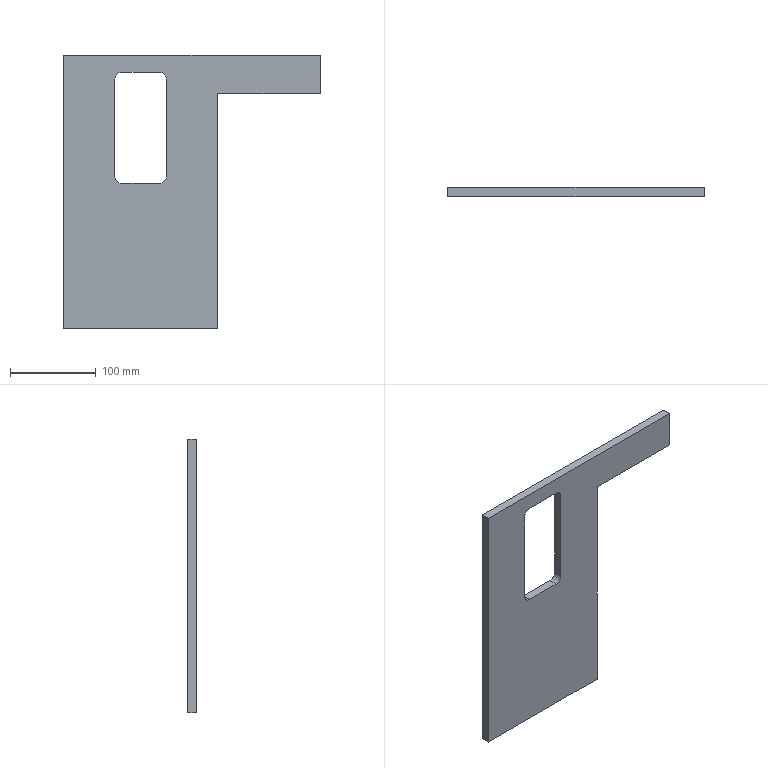Part | SolidWorks | features Cut 1, Extrusion 1, Fillet 1, ICE 1 | 1 solid | 16 faces | box 300 x 10 x 320 mm | volume 552549 mm3 | plane 12 | cylinder 4 | commonest cylinder face diameters 16 x4
STEP:
#1=CARTESIAN_POINT('',(90.,0.,115.));
#2=VERTEX_POINT('',#1);
#3=CARTESIAN_POINT('',(90.,10.,115.));
#4=VERTEX_POINT('',#3);
#5=CARTESIAN_POINT('',(90.,10.,115.));
#6=DIRECTION('',(0.,1.,0.));
#7=VECTOR('',#6,1000.);
#8=LINE('',#5,#7);
#9=EDGE_CURVE('',#2,#4,#8,.T.);
#10=ORIENTED_EDGE('',*,*,#9,.F.);
#11=CARTESIAN_POINT('',(90.,0.,-160.));
#12=VERTEX_POINT('',#11);
#13=CARTESIAN_POINT('',(90.,0.,-160.));
#14=DIRECTION('',(0.,0.,-1.));
#15=VECTOR('',#14,1000.);
#16=LINE('',#13,#15);
#17=EDGE_CURVE('',#2,#12,#16,.T.);
#18=ORIENTED_EDGE('',*,*,#17,.T.);
#19=CARTESIAN_POINT('',(90.,10.,-160.));
#20=VERTEX_POINT('',#19);
#21=CARTESIAN_POINT('',(90.,10.,-160.));
#22=DIRECTION('',(0.,-1.,0.));
#23=VECTOR('',#22,1000.);
#24=LINE('',#21,#23);
#25=EDGE_CURVE('',#20,#12,#24,.T.);
#26=ORIENTED_EDGE('',*,*,#25,.F.);
#27=CARTESIAN_POINT('',(90.,10.,-160.));
#28=DIRECTION('',(0.,0.,-1.));
#29=VECTOR('',#28,1000.);
#30=LINE('',#27,#29);
#31=EDGE_CURVE('',#4,#20,#30,.T.);
#32=ORIENTED_EDGE('',*,*,#31,.F.);
#33=EDGE_LOOP('',(#10,#18,#26,#32));
#34=FACE_OUTER_BOUND('',#33,.T.);
#35=CARTESIAN_POINT('',(90.,10.,-160.));
#36=DIRECTION('',(-1.,0.,0.));
#37=DIRECTION('',(0.,0.,1.));
#38=AXIS2_PLACEMENT_3D('',#35,#36,#37);
#39=PLANE('',#38);
#40=ADVANCED_FACE('',(#34),#39,.F.);
#41=CARTESIAN_POINT('',(-90.,0.,-160.));
#42=VERTEX_POINT('',#41);
#43=CARTESIAN_POINT('',(-90.,0.,-160.));
#44=DIRECTION('',(-1.,0.,0.));
#45=VECTOR('',#44,1000.);
#46=LINE('',#43,#45);
#47=EDGE_CURVE('',#12,#42,#46,.T.);
#48=ORIENTED_EDGE('',*,*,#47,.T.);
#49=CARTESIAN_POINT('',(-90.,10.,-160.));
#50=VERTEX_POINT('',#49);
#51=CARTESIAN_POINT('',(-90.,10.,-160.));
#52=DIRECTION('',(0.,-1.,0.));
#53=VECTOR('',#52,1000.);
#54=LINE('',#51,#53);
#55=EDGE_CURVE('',#50,#42,#54,.T.);
#56=ORIENTED_EDGE('',*,*,#55,.F.);
#57=CARTESIAN_POINT('',(-90.,10.,-160.));
#58=DIRECTION('',(-1.,0.,0.));
#59=VECTOR('',#58,1000.);
#60=LINE('',#57,#59);
#61=EDGE_CURVE('',#20,#50,#60,.T.);
#62=ORIENTED_EDGE('',*,*,#61,.F.);
#63=ORIENTED_EDGE('',*,*,#25,.T.);
#64=EDGE_LOOP('',(#48,#56,#62,#63));
#65=FACE_OUTER_BOUND('',#64,.T.);
#66=CARTESIAN_POINT('',(-90.,10.,-160.));
#67=DIRECTION('',(0.,0.,1.));
#68=DIRECTION('',(1.,0.,0.));
#69=AXIS2_PLACEMENT_3D('',#66,#67,#68);
#70=PLANE('',#69);
#71=ADVANCED_FACE('',(#65),#70,.F.);
#72=CARTESIAN_POINT('',(-90.,0.,160.));
#73=VERTEX_POINT('',#72);
#74=CARTESIAN_POINT('',(-90.,0.,-160.));
#75=DIRECTION('',(0.,0.,1.));
#76=VECTOR('',#75,1000.);
#77=LINE('',#74,#76);
#78=EDGE_CURVE('',#42,#73,#77,.T.);
#79=ORIENTED_EDGE('',*,*,#78,.T.);
#80=CARTESIAN_POINT('',(-90.,10.,160.));
#81=VERTEX_POINT('',#80);
#82=CARTESIAN_POINT('',(-90.,10.,160.));
#83=DIRECTION('',(0.,-1.,0.));
#84=VECTOR('',#83,1000.);
#85=LINE('',#82,#84);
#86=EDGE_CURVE('',#81,#73,#85,.T.);
#87=ORIENTED_EDGE('',*,*,#86,.F.);
#88=CARTESIAN_POINT('',(-90.,10.,-160.));
#89=DIRECTION('',(0.,0.,1.));
#90=VECTOR('',#89,1000.);
#91=LINE('',#88,#90);
#92=EDGE_CURVE('',#50,#81,#91,.T.);
#93=ORIENTED_EDGE('',*,*,#92,.F.);
#94=ORIENTED_EDGE('',*,*,#55,.T.);
#95=EDGE_LOOP('',(#79,#87,#93,#94));
#96=FACE_OUTER_BOUND('',#95,.T.);
#97=CARTESIAN_POINT('',(-90.,10.,-160.));
#98=DIRECTION('',(1.,0.,0.));
#99=DIRECTION('',(0.,0.,-1.));
#100=AXIS2_PLACEMENT_3D('',#97,#98,#99);
#101=PLANE('',#100);
#102=ADVANCED_FACE('',(#96),#101,.F.);
#103=CARTESIAN_POINT('',(210.,0.,160.));
#104=VERTEX_POINT('',#103);
#105=CARTESIAN_POINT('',(-90.,0.,160.));
#106=DIRECTION('',(1.,0.,0.));
#107=VECTOR('',#106,1000.);
#108=LINE('',#105,#107);
#109=EDGE_CURVE('',#73,#104,#108,.T.);
#110=ORIENTED_EDGE('',*,*,#109,.T.);
#111=CARTESIAN_POINT('',(210.,10.,160.));
#112=VERTEX_POINT('',#111);
#113=CARTESIAN_POINT('',(210.,10.,160.));
#114=DIRECTION('',(0.,-1.,0.));
#115=VECTOR('',#114,1000.);
#116=LINE('',#113,#115);
#117=EDGE_CURVE('',#112,#104,#116,.T.);
#118=ORIENTED_EDGE('',*,*,#117,.F.);
#119=CARTESIAN_POINT('',(-90.,10.,160.));
#120=DIRECTION('',(1.,0.,0.));
#121=VECTOR('',#120,1000.);
#122=LINE('',#119,#121);
#123=EDGE_CURVE('',#81,#112,#122,.T.);
#124=ORIENTED_EDGE('',*,*,#123,.F.);
#125=ORIENTED_EDGE('',*,*,#86,.T.);
#126=EDGE_LOOP('',(#110,#118,#124,#125));
#127=FACE_OUTER_BOUND('',#126,.T.);
#128=CARTESIAN_POINT('',(-90.,10.,160.));
#129=DIRECTION('',(0.,0.,-1.));
#130=DIRECTION('',(-1.,0.,0.));
#131=AXIS2_PLACEMENT_3D('',#128,#129,#130);
#132=PLANE('',#131);
#133=ADVANCED_FACE('',(#127),#132,.F.);
#134=CARTESIAN_POINT('',(30.,10.,132.));
#135=VERTEX_POINT('',#134);
#136=CARTESIAN_POINT('',(30.,10.,18.));
#137=VERTEX_POINT('',#136);
#138=CARTESIAN_POINT('',(30.,10.,10.));
#139=DIRECTION('',(0.,0.,-1.));
#140=VECTOR('',#139,1000.);
#141=LINE('',#138,#140);
#142=EDGE_CURVE('',#135,#137,#141,.T.);
#143=ORIENTED_EDGE('',*,*,#142,.F.);
#144=CARTESIAN_POINT('',(22.,10.,140.));
#145=VERTEX_POINT('',#144);
#146=CARTESIAN_POINT('',(22.,10.,132.));
#147=DIRECTION('',(0.,-1.,0.));
#148=DIRECTION('',(0.,0.,1.));
#149=AXIS2_PLACEMENT_3D('',#146,#147,#148);
#150=CIRCLE('',#149,8.);
#151=EDGE_CURVE('',#135,#145,#150,.T.);
#152=ORIENTED_EDGE('',*,*,#151,.T.);
#153=CARTESIAN_POINT('',(-22.,10.,140.));
#154=VERTEX_POINT('',#153);
#155=CARTESIAN_POINT('',(30.,10.,140.));
#156=DIRECTION('',(1.,0.,0.));
#157=VECTOR('',#156,1000.);
#158=LINE('',#155,#157);
#159=EDGE_CURVE('',#154,#145,#158,.T.);
#160=ORIENTED_EDGE('',*,*,#159,.F.);
#161=CARTESIAN_POINT('',(-30.,10.,132.));
#162=VERTEX_POINT('',#161);
#163=CARTESIAN_POINT('',(-22.,10.,132.));
#164=DIRECTION('',(0.,-1.,0.));
#165=DIRECTION('',(0.,0.,1.));
#166=AXIS2_PLACEMENT_3D('',#163,#164,#165);
#167=CIRCLE('',#166,8.);
#168=EDGE_CURVE('',#154,#162,#167,.T.);
#169=ORIENTED_EDGE('',*,*,#168,.T.);
#170=CARTESIAN_POINT('',(-30.,10.,18.));
#171=VERTEX_POINT('',#170);
#172=CARTESIAN_POINT('',(-30.,10.,10.));
#173=DIRECTION('',(0.,0.,1.));
#174=VECTOR('',#173,1000.);
#175=LINE('',#172,#174);
#176=EDGE_CURVE('',#171,#162,#175,.T.);
#177=ORIENTED_EDGE('',*,*,#176,.F.);
#178=CARTESIAN_POINT('',(-22.,10.,10.));
#179=VERTEX_POINT('',#178);
#180=CARTESIAN_POINT('',(-22.,10.,18.));
#181=DIRECTION('',(0.,-1.,0.));
#182=DIRECTION('',(0.,0.,1.));
#183=AXIS2_PLACEMENT_3D('',#180,#181,#182);
#184=CIRCLE('',#183,8.);
#185=EDGE_CURVE('',#171,#179,#184,.T.);
#186=ORIENTED_EDGE('',*,*,#185,.T.);
#187=CARTESIAN_POINT('',(22.,10.,10.));
#188=VERTEX_POINT('',#187);
#189=CARTESIAN_POINT('',(30.,10.,10.));
#190=DIRECTION('',(-1.,0.,0.));
#191=VECTOR('',#190,1000.);
#192=LINE('',#189,#191);
#193=EDGE_CURVE('',#188,#179,#192,.T.);
#194=ORIENTED_EDGE('',*,*,#193,.F.);
#195=CARTESIAN_POINT('',(22.,10.,18.));
#196=DIRECTION('',(0.,-1.,0.));
#197=DIRECTION('',(0.,0.,1.));
#198=AXIS2_PLACEMENT_3D('',#195,#196,#197);
#199=CIRCLE('',#198,8.);
#200=EDGE_CURVE('',#188,#137,#199,.T.);
#201=ORIENTED_EDGE('',*,*,#200,.T.);
#202=EDGE_LOOP('',(#143,#152,#160,#169,#177,#186,#194,#201));
#203=FACE_BOUND('',#202,.T.);
#204=ORIENTED_EDGE('',*,*,#123,.T.);
#205=CARTESIAN_POINT('',(210.,10.,115.));
#206=VERTEX_POINT('',#205);
#207=CARTESIAN_POINT('',(210.,10.,160.));
#208=DIRECTION('',(0.,0.,1.));
#209=VECTOR('',#208,1000.);
#210=LINE('',#207,#209);
#211=EDGE_CURVE('',#206,#112,#210,.T.);
#212=ORIENTED_EDGE('',*,*,#211,.F.);
#213=CARTESIAN_POINT('',(210.,10.,115.));
#214=DIRECTION('',(-1.,0.,0.));
#215=VECTOR('',#214,1000.);
#216=LINE('',#213,#215);
#217=EDGE_CURVE('',#206,#4,#216,.T.);
#218=ORIENTED_EDGE('',*,*,#217,.T.);
#219=ORIENTED_EDGE('',*,*,#31,.T.);
#220=ORIENTED_EDGE('',*,*,#61,.T.);
#221=ORIENTED_EDGE('',*,*,#92,.T.);
#222=EDGE_LOOP('',(#204,#212,#218,#219,#220,#221));
#223=FACE_OUTER_BOUND('',#222,.T.);
#224=CARTESIAN_POINT('',(0.,10.,0.));
#225=DIRECTION('',(0.,1.,0.));
#226=DIRECTION('',(0.,0.,1.));
#227=AXIS2_PLACEMENT_3D('',#224,#225,#226);
#228=PLANE('',#227);
#229=ADVANCED_FACE('',(#203,#223),#228,.T.);
#230=CARTESIAN_POINT('',(-30.,0.,18.));
#231=VERTEX_POINT('',#230);
#232=CARTESIAN_POINT('',(-30.,0.,132.));
#233=VERTEX_POINT('',#232);
#234=CARTESIAN_POINT('',(-30.,0.,10.));
#235=DIRECTION('',(0.,0.,1.));
#236=VECTOR('',#235,1000.);
#237=LINE('',#234,#236);
#238=EDGE_CURVE('',#231,#233,#237,.T.);
#239=ORIENTED_EDGE('',*,*,#238,.T.);
#240=CARTESIAN_POINT('',(-22.,0.,140.));
#241=VERTEX_POINT('',#240);
#242=CARTESIAN_POINT('',(-22.,0.,132.));
#243=DIRECTION('',(0.,1.,0.));
#244=DIRECTION('',(0.,0.,1.));
#245=AXIS2_PLACEMENT_3D('',#242,#243,#244);
#246=CIRCLE('',#245,8.);
#247=EDGE_CURVE('',#233,#241,#246,.T.);
#248=ORIENTED_EDGE('',*,*,#247,.T.);
#249=CARTESIAN_POINT('',(22.,0.,140.));
#250=VERTEX_POINT('',#249);
#251=CARTESIAN_POINT('',(30.,0.,140.));
#252=DIRECTION('',(1.,0.,0.));
#253=VECTOR('',#252,1000.);
#254=LINE('',#251,#253);
#255=EDGE_CURVE('',#241,#250,#254,.T.);
#256=ORIENTED_EDGE('',*,*,#255,.T.);
#257=CARTESIAN_POINT('',(30.,0.,132.));
#258=VERTEX_POINT('',#257);
#259=CARTESIAN_POINT('',(22.,0.,132.));
#260=DIRECTION('',(0.,1.,0.));
#261=DIRECTION('',(0.,0.,1.));
#262=AXIS2_PLACEMENT_3D('',#259,#260,#261);
#263=CIRCLE('',#262,8.);
#264=EDGE_CURVE('',#250,#258,#263,.T.);
#265=ORIENTED_EDGE('',*,*,#264,.T.);
#266=CARTESIAN_POINT('',(30.,0.,18.));
#267=VERTEX_POINT('',#266);
#268=CARTESIAN_POINT('',(30.,0.,10.));
#269=DIRECTION('',(0.,0.,-1.));
#270=VECTOR('',#269,1000.);
#271=LINE('',#268,#270);
#272=EDGE_CURVE('',#258,#267,#271,.T.);
#273=ORIENTED_EDGE('',*,*,#272,.T.);
#274=CARTESIAN_POINT('',(22.,0.,10.));
#275=VERTEX_POINT('',#274);
#276=CARTESIAN_POINT('',(22.,0.,18.));
#277=DIRECTION('',(0.,1.,0.));
#278=DIRECTION('',(0.,0.,1.));
#279=AXIS2_PLACEMENT_3D('',#276,#277,#278);
#280=CIRCLE('',#279,8.);
#281=EDGE_CURVE('',#267,#275,#280,.T.);
#282=ORIENTED_EDGE('',*,*,#281,.T.);
#283=CARTESIAN_POINT('',(-22.,0.,10.));
#284=VERTEX_POINT('',#283);
#285=CARTESIAN_POINT('',(30.,0.,10.));
#286=DIRECTION('',(-1.,0.,0.));
#287=VECTOR('',#286,1000.);
#288=LINE('',#285,#287);
#289=EDGE_CURVE('',#275,#284,#288,.T.);
#290=ORIENTED_EDGE('',*,*,#289,.T.);
#291=CARTESIAN_POINT('',(-22.,0.,18.));
#292=DIRECTION('',(0.,1.,0.));
#293=DIRECTION('',(0.,0.,1.));
#294=AXIS2_PLACEMENT_3D('',#291,#292,#293);
#295=CIRCLE('',#294,8.);
#296=EDGE_CURVE('',#284,#231,#295,.T.);
#297=ORIENTED_EDGE('',*,*,#296,.T.);
#298=EDGE_LOOP('',(#239,#248,#256,#265,#273,#282,#290,#297));
#299=FACE_BOUND('',#298,.T.);
#300=ORIENTED_EDGE('',*,*,#17,.F.);
#301=CARTESIAN_POINT('',(210.,0.,115.));
#302=VERTEX_POINT('',#301);
#303=CARTESIAN_POINT('',(210.,0.,115.));
#304=DIRECTION('',(-1.,0.,0.));
#305=VECTOR('',#304,1000.);
#306=LINE('',#303,#305);
#307=EDGE_CURVE('',#302,#2,#306,.T.);
#308=ORIENTED_EDGE('',*,*,#307,.F.);
#309=CARTESIAN_POINT('',(210.,0.,160.));
#310=DIRECTION('',(0.,0.,-1.));
#311=VECTOR('',#310,1000.);
#312=LINE('',#309,#311);
#313=EDGE_CURVE('',#104,#302,#312,.T.);
#314=ORIENTED_EDGE('',*,*,#313,.F.);
#315=ORIENTED_EDGE('',*,*,#109,.F.);
#316=ORIENTED_EDGE('',*,*,#78,.F.);
#317=ORIENTED_EDGE('',*,*,#47,.F.);
#318=EDGE_LOOP('',(#300,#308,#314,#315,#316,#317));
#319=FACE_OUTER_BOUND('',#318,.T.);
#320=CARTESIAN_POINT('',(0.,0.,0.));
#321=DIRECTION('',(0.,1.,0.));
#322=DIRECTION('',(0.,0.,1.));
#323=AXIS2_PLACEMENT_3D('',#320,#321,#322);
#324=PLANE('',#323);
#325=ADVANCED_FACE('',(#299,#319),#324,.F.);
#326=ORIENTED_EDGE('',*,*,#272,.F.);
#327=CARTESIAN_POINT('',(30.,10.,132.));
#328=DIRECTION('',(0.,1.,0.));
#329=VECTOR('',#328,1000.);
#330=LINE('',#327,#329);
#331=EDGE_CURVE('',#258,#135,#330,.T.);
#332=ORIENTED_EDGE('',*,*,#331,.T.);
#333=ORIENTED_EDGE('',*,*,#142,.T.);
#334=CARTESIAN_POINT('',(30.,0.,18.));
#335=DIRECTION('',(0.,-1.,0.));
#336=VECTOR('',#335,1000.);
#337=LINE('',#334,#336);
#338=EDGE_CURVE('',#137,#267,#337,.T.);
#339=ORIENTED_EDGE('',*,*,#338,.T.);
#340=EDGE_LOOP('',(#326,#332,#333,#339));
#341=FACE_OUTER_BOUND('',#340,.T.);
#342=CARTESIAN_POINT('',(30.,0.,10.));
#343=DIRECTION('',(1.,0.,0.));
#344=DIRECTION('',(0.,0.,-1.));
#345=AXIS2_PLACEMENT_3D('',#342,#343,#344);
#346=PLANE('',#345);
#347=ADVANCED_FACE('',(#341),#346,.F.);
#348=ORIENTED_EDGE('',*,*,#159,.T.);
#349=CARTESIAN_POINT('',(22.,0.,140.));
#350=DIRECTION('',(0.,-1.,0.));
#351=VECTOR('',#350,1000.);
#352=LINE('',#349,#351);
#353=EDGE_CURVE('',#145,#250,#352,.T.);
#354=ORIENTED_EDGE('',*,*,#353,.T.);
#355=ORIENTED_EDGE('',*,*,#255,.F.);
#356=CARTESIAN_POINT('',(-22.,10.,140.));
#357=DIRECTION('',(0.,1.,0.));
#358=VECTOR('',#357,1000.);
#359=LINE('',#356,#358);
#360=EDGE_CURVE('',#241,#154,#359,.T.);
#361=ORIENTED_EDGE('',*,*,#360,.T.);
#362=EDGE_LOOP('',(#348,#354,#355,#361));
#363=FACE_OUTER_BOUND('',#362,.T.);
#364=CARTESIAN_POINT('',(30.,0.,140.));
#365=DIRECTION('',(0.,0.,1.));
#366=DIRECTION('',(1.,0.,0.));
#367=AXIS2_PLACEMENT_3D('',#364,#365,#366);
#368=PLANE('',#367);
#369=ADVANCED_FACE('',(#363),#368,.F.);
#370=ORIENTED_EDGE('',*,*,#176,.T.);
#371=CARTESIAN_POINT('',(-30.,0.,132.));
#372=DIRECTION('',(0.,-1.,0.));
#373=VECTOR('',#372,1000.);
#374=LINE('',#371,#373);
#375=EDGE_CURVE('',#162,#233,#374,.T.);
#376=ORIENTED_EDGE('',*,*,#375,.T.);
#377=ORIENTED_EDGE('',*,*,#238,.F.);
#378=CARTESIAN_POINT('',(-30.,10.,18.));
#379=DIRECTION('',(0.,1.,0.));
#380=VECTOR('',#379,1000.);
#381=LINE('',#378,#380);
#382=EDGE_CURVE('',#231,#171,#381,.T.);
#383=ORIENTED_EDGE('',*,*,#382,.T.);
#384=EDGE_LOOP('',(#370,#376,#377,#383));
#385=FACE_OUTER_BOUND('',#384,.T.);
#386=CARTESIAN_POINT('',(-30.,0.,10.));
#387=DIRECTION('',(-1.,0.,0.));
#388=DIRECTION('',(0.,0.,1.));
#389=AXIS2_PLACEMENT_3D('',#386,#387,#388);
#390=PLANE('',#389);
#391=ADVANCED_FACE('',(#385),#390,.F.);
#392=ORIENTED_EDGE('',*,*,#193,.T.);
#393=CARTESIAN_POINT('',(-22.,0.,10.));
#394=DIRECTION('',(0.,-1.,0.));
#395=VECTOR('',#394,1000.);
#396=LINE('',#393,#395);
#397=EDGE_CURVE('',#179,#284,#396,.T.);
#398=ORIENTED_EDGE('',*,*,#397,.T.);
#399=ORIENTED_EDGE('',*,*,#289,.F.);
#400=CARTESIAN_POINT('',(22.,10.,10.));
#401=DIRECTION('',(0.,1.,0.));
#402=VECTOR('',#401,1000.);
#403=LINE('',#400,#402);
#404=EDGE_CURVE('',#275,#188,#403,.T.);
#405=ORIENTED_EDGE('',*,*,#404,.T.);
#406=EDGE_LOOP('',(#392,#398,#399,#405));
#407=FACE_OUTER_BOUND('',#406,.T.);
#408=CARTESIAN_POINT('',(30.,0.,10.));
#409=DIRECTION('',(0.,0.,-1.));
#410=DIRECTION('',(-1.,0.,0.));
#411=AXIS2_PLACEMENT_3D('',#408,#409,#410);
#412=PLANE('',#411);
#413=ADVANCED_FACE('',(#407),#412,.F.);
#414=ORIENTED_EDGE('',*,*,#264,.F.);
#415=ORIENTED_EDGE('',*,*,#353,.F.);
#416=ORIENTED_EDGE('',*,*,#151,.F.);
#417=ORIENTED_EDGE('',*,*,#331,.F.);
#418=EDGE_LOOP('',(#414,#415,#416,#417));
#419=FACE_OUTER_BOUND('',#418,.T.);
#420=CARTESIAN_POINT('',(22.,0.,132.));
#421=DIRECTION('',(0.,-1.,0.));
#422=DIRECTION('',(0.,0.,-1.));
#423=AXIS2_PLACEMENT_3D('',#420,#421,#422);
#424=CYLINDRICAL_SURFACE('',#423,8.);
#425=ADVANCED_FACE('',(#419),#424,.F.);
#426=ORIENTED_EDGE('',*,*,#247,.F.);
#427=ORIENTED_EDGE('',*,*,#375,.F.);
#428=ORIENTED_EDGE('',*,*,#168,.F.);
#429=ORIENTED_EDGE('',*,*,#360,.F.);
#430=EDGE_LOOP('',(#426,#427,#428,#429));
#431=FACE_OUTER_BOUND('',#430,.T.);
#432=CARTESIAN_POINT('',(-22.,0.,132.));
#433=DIRECTION('',(0.,-1.,0.));
#434=DIRECTION('',(0.,0.,-1.));
#435=AXIS2_PLACEMENT_3D('',#432,#433,#434);
#436=CYLINDRICAL_SURFACE('',#435,8.);
#437=ADVANCED_FACE('',(#431),#436,.F.);
#438=ORIENTED_EDGE('',*,*,#296,.F.);
#439=ORIENTED_EDGE('',*,*,#397,.F.);
#440=ORIENTED_EDGE('',*,*,#185,.F.);
#441=ORIENTED_EDGE('',*,*,#382,.F.);
#442=EDGE_LOOP('',(#438,#439,#440,#441));
#443=FACE_OUTER_BOUND('',#442,.T.);
#444=CARTESIAN_POINT('',(-22.,0.,18.));
#445=DIRECTION('',(0.,-1.,0.));
#446=DIRECTION('',(0.,0.,-1.));
#447=AXIS2_PLACEMENT_3D('',#444,#445,#446);
#448=CYLINDRICAL_SURFACE('',#447,8.);
#449=ADVANCED_FACE('',(#443),#448,.F.);
#450=ORIENTED_EDGE('',*,*,#281,.F.);
#451=ORIENTED_EDGE('',*,*,#338,.F.);
#452=ORIENTED_EDGE('',*,*,#200,.F.);
#453=ORIENTED_EDGE('',*,*,#404,.F.);
#454=EDGE_LOOP('',(#450,#451,#452,#453));
#455=FACE_OUTER_BOUND('',#454,.T.);
#456=CARTESIAN_POINT('',(22.,0.,18.));
#457=DIRECTION('',(0.,-1.,0.));
#458=DIRECTION('',(0.,0.,-1.));
#459=AXIS2_PLACEMENT_3D('',#456,#457,#458);
#460=CYLINDRICAL_SURFACE('',#459,8.);
#461=ADVANCED_FACE('',(#455),#460,.F.);
#462=ORIENTED_EDGE('',*,*,#9,.T.);
#463=ORIENTED_EDGE('',*,*,#217,.F.);
#464=CARTESIAN_POINT('',(210.,10.,115.));
#465=DIRECTION('',(0.,1.,0.));
#466=VECTOR('',#465,1000.);
#467=LINE('',#464,#466);
#468=EDGE_CURVE('',#302,#206,#467,.T.);
#469=ORIENTED_EDGE('',*,*,#468,.F.);
#470=ORIENTED_EDGE('',*,*,#307,.T.);
#471=EDGE_LOOP('',(#462,#463,#469,#470));
#472=FACE_OUTER_BOUND('',#471,.T.);
#473=CARTESIAN_POINT('',(210.,10.,115.));
#474=DIRECTION('',(0.,0.,1.));
#475=DIRECTION('',(1.,0.,0.));
#476=AXIS2_PLACEMENT_3D('',#473,#474,#475);
#477=PLANE('',#476);
#478=ADVANCED_FACE('',(#472),#477,.F.);
#479=ORIENTED_EDGE('',*,*,#117,.T.);
#480=ORIENTED_EDGE('',*,*,#313,.T.);
#481=ORIENTED_EDGE('',*,*,#468,.T.);
#482=ORIENTED_EDGE('',*,*,#211,.T.);
#483=EDGE_LOOP('',(#479,#480,#481,#482));
#484=FACE_OUTER_BOUND('',#483,.T.);
#485=CARTESIAN_POINT('',(210.,0.,0.));
#486=DIRECTION('',(1.,0.,0.));
#487=DIRECTION('',(0.,0.,-1.));
#488=AXIS2_PLACEMENT_3D('',#485,#486,#487);
#489=PLANE('',#488);
#490=ADVANCED_FACE('',(#484),#489,.T.);
#491=CLOSED_SHELL('',(#40,#71,#102,#133,#229,#325,#347,#369,#391,#413,#425,#437,#449,#461,#478,#490));
#492=MANIFOLD_SOLID_BREP('',#491);
#493=CARTESIAN_POINT('',(0.,0.,0.));
#494=DIRECTION('',(0.,0.,1.));
#495=DIRECTION('',(1.,0.,0.));
#496=AXIS2_PLACEMENT_3D('',#493,#494,#495);
#497=(LENGTH_UNIT()NAMED_UNIT(*)SI_UNIT(.MILLI.,.METRE.));
#498=UNCERTAINTY_MEASURE_WITH_UNIT(LENGTH_MEASURE(0.00001),#497,'','');
#499=(NAMED_UNIT(*)PLANE_ANGLE_UNIT()SI_UNIT($,.RADIAN.));
#500=(NAMED_UNIT(*)SI_UNIT($,.STERADIAN.)SOLID_ANGLE_UNIT());
#501=(GEOMETRIC_REPRESENTATION_CONTEXT(3)GLOBAL_UNCERTAINTY_ASSIGNED_CONTEXT((#498))GLOBAL_UNIT_ASSIGNED_CONTEXT((#497,#499,#500))REPRESENTATION_CONTEXT('',''));
#502=ADVANCED_BREP_SHAPE_REPRESENTATION('',(#492,#496),#501);